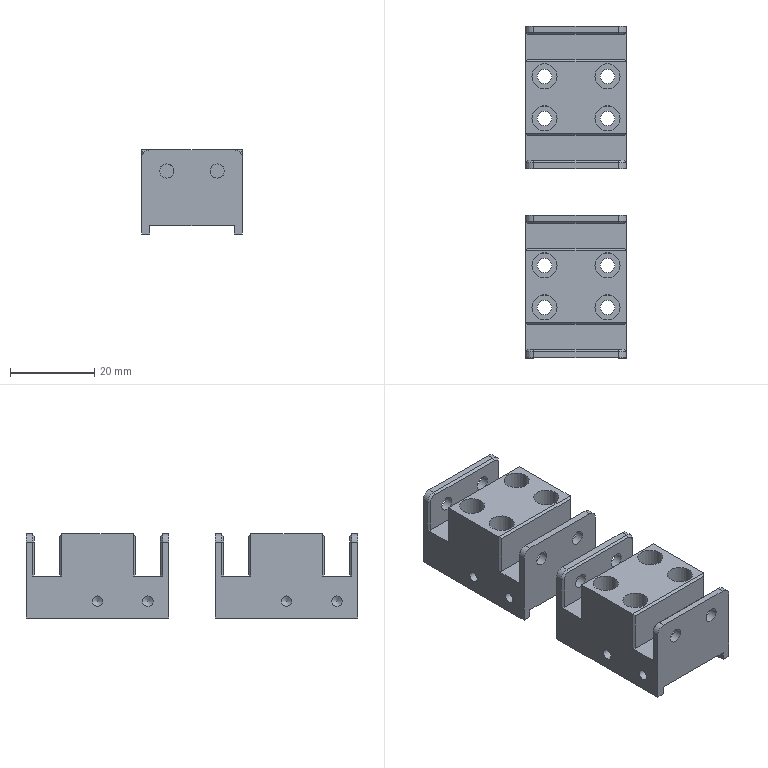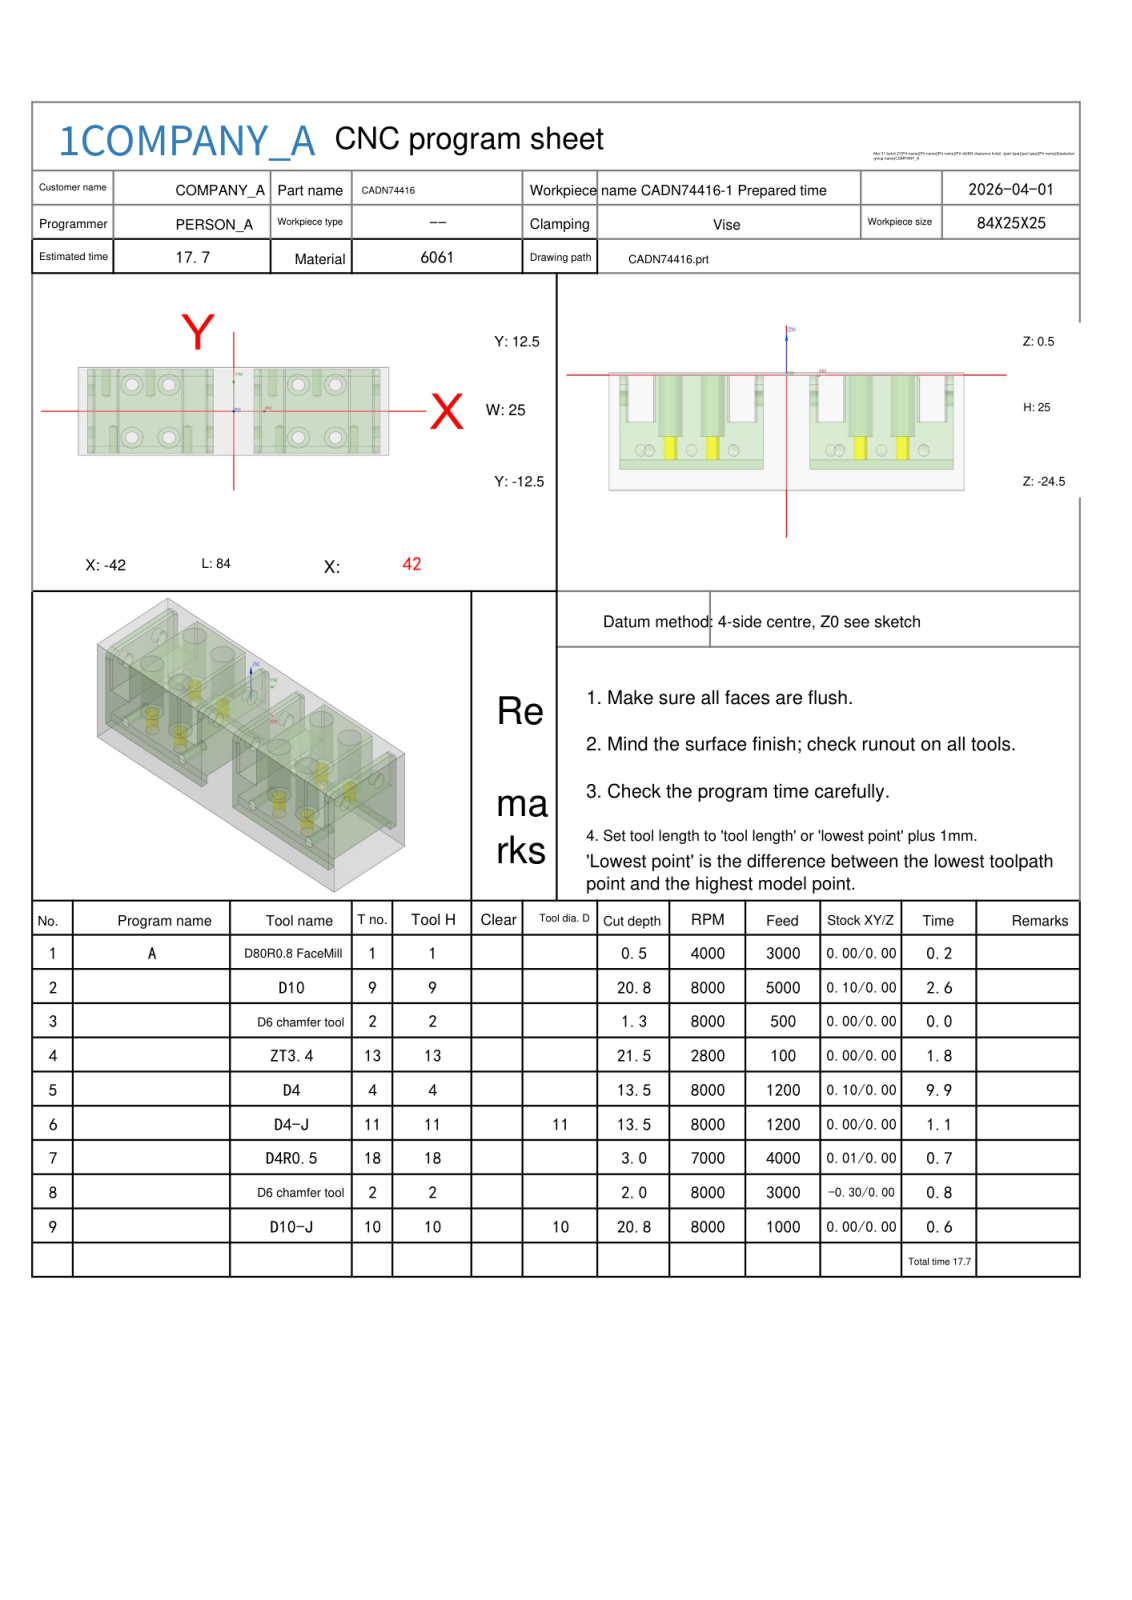NC program | NX | posted by the shop | part box 24 x 79 x 20 mm
Lines 7104 to 7697 of 7697:
N8 T02 M06
(D6 chamfer tool  D=6. R=0. H=02 ce=0.00 di=0.00)
G00 G90 G54 X41.628 Y10.25 M03 S8000
G43 H02 Z20.
M08
Z2.085
G01 Z-1.5 F3000.
G03 X41.328 Y10.33 I-.3 J-.52
X40.808 Y10.03 I0.0 J-.6
G01 X40.8 Y10.
Y-10.
X40.808 Y-10.03
G03 X41.328 Y-10.33 I.52 J.3
X41.628 Y-10.25 I0.0 J.6
G01 Z2.085
G00 Z3.45
X32.171 Y-12.564
Z2.927
G01 Z-1.5
G02 X31. Y-13.3 I-1.171 J.564
G01 X14.
G02 X12.829 Y-12.564 I0.0 J1.3
G01 Z2.927
G00 Z20.
Y12.564
Z2.927
G01 Z-1.5
G02 X14. Y13.3 I1.171 J-.564
G01 X31.
G02 X32.171 Y12.564 I0.0 J-1.3
G01 Z2.927
G00 Z20.
X3.372 Y-10.25
Z2.085
G01 Z-1.5
G03 X3.672 Y-10.33 I.3 J.52
X4.192 Y-10.03 I0.0 J.6
G01 X4.2 Y-10.
Y10.
X4.192 Y10.03
G03 X3.672 Y10.33 I-.52 J-.3
X3.372 Y10.25 I0.0 J-.6
G01 Z2.085
G00 Z2.25
X-3.372
Z2.085
G01 Z-1.5
G03 X-3.672 Y10.33 I-.3 J-.52
X-4.192 Y10.03 I0.0 J-.6
G01 X-4.2 Y10.
Y-10.
X-4.192 Y-10.03
G03 X-3.672 Y-10.33 I.52 J.3
X-3.372 Y-10.25 I0.0 J.6
G01 Z2.085
G00 Z3.45
X-12.829 Y-12.564
Z2.927
G01 Z-1.5
G02 X-14. Y-13.3 I-1.171 J.564
G01 X-31.
G02 X-32.171 Y-12.564 I0.0 J1.3
G01 Z2.927
G00 Z20.
Y12.564
Z2.927
G01 Z-1.5
G02 X-31. Y13.3 I1.171 J-.564
G01 X-14.
G02 X-12.829 Y12.564 I0.0 J-1.3
G01 Z2.927
G00 Z20.
X-41.628 Y-10.25
Z2.085
G01 Z-1.5
G03 X-41.328 Y-10.33 I.3 J.52
X-40.808 Y-10.03 I0.0 J.6
G01 X-40.8 Y-10.
Y10.
X-40.808 Y10.03
G03 X-41.328 Y10.33 I-.52 J-.3
X-41.628 Y10.25 I0.0 J-.6
G01 Z2.085
G00 Z20.
G00 G90 X-36.706 Y13.228 M03 S6500
Z20.
Z.3
G01 Z-1.2 F1500.
G03 X-36.8 Y12.763 I1.106 J-.465
G01 Y10.142
G03 X-35.6 Y8.942 I1.2 J0.0
G01 Y11.2
G03 X-36.8 Y10. I0.0 J-1.2
G01 Y-10.
G03 X-35.6 Y-11.2 I1.2 J0.0
G01 Y-8.942
G03 X-36.8 Y-10.142 I0.0 J-1.2
G01 Y-12.763
G03 X-36.706 Y-13.228 I1.2 J0.0
G01 Z.3
G00 Z20.
X-8.294
Z.3
G01 Z-1.2
G03 X-8.2 Y-12.763 I-1.106 J.465
G01 Y-10.142
G03 X-9.4 Y-8.942 I-1.2 J0.0
G01 Y-11.2
G03 X-8.2 Y-10. I0.0 J1.2
G01 Y10.
G03 X-9.4 Y11.2 I-1.2 J0.0
G01 Y8.942
G03 X-8.2 Y10.142 I0.0 J1.2
G01 Y12.763
G03 X-8.294 Y13.228 I-1.2 J0.0
G01 Z.3
G00 Z20.
X8.294
Z.3
G01 Z-1.2
G03 X8.2 Y12.763 I1.106 J-.465
G01 Y10.142
G03 X9.4 Y8.942 I1.2 J0.0
G01 Y11.2
G03 X8.2 Y10. I0.0 J-1.2
G01 Y-10.
G03 X9.4 Y-11.2 I1.2 J0.0
G01 Y-8.942
G03 X8.2 Y-10.142 I0.0 J-1.2
G01 Y-12.763
G03 X8.294 Y-13.228 I1.2 J0.0
G01 Z.3
G00 Z20.
X36.706
Z.3
G01 Z-1.2
G03 X36.8 Y-12.763 I-1.106 J.465
G01 Y-10.142
G03 X35.6 Y-8.942 I-1.2 J0.0
G01 Y-11.2
G03 X36.8 Y-10. I0.0 J1.2
G01 Y10.
G03 X35.6 Y11.2 I-1.2 J0.0
G01 Y8.942
G03 X36.8 Y10.142 I0.0 J1.2
G01 Y12.763
G03 X36.706 Y13.228 I-1.2 J0.0
G01 Z.3
G00 Z20.
G00 G90 X-15.519 Y8.67 M03 S8000
Z20.
Z2.5
G01 X-15.567 Y8.752 Z2.465 F500.
X-15.764 Y9.013 Z2.346
X-15.996 Y9.244 Z2.227
X-16.259 Y9.44 Z2.108
X-16.546 Y9.596 Z1.989
X-16.853 Y9.71 Z1.87
X-17.173 Y9.78 Z1.75
X-17.5 Y9.803 Z1.631
X-17.827 Y9.78 Z1.512
X-18.147 Y9.71 Z1.393
X-18.454 Y9.596 Z1.274
X-18.741 Y9.44 Z1.154
X-19.004 Y9.244 Z1.035
X-19.236 Y9.013 Z.916
X-19.433 Y8.752 Z.797
X-19.551 Y8.548 Z.711
X-19.679 Y8.247 Z.592
X-19.762 Y7.93 Z.473
X-19.801 Y7.605 Z.354
X-19.792 Y7.278 Z.235
X-19.738 Y6.955 Z.115
X-19.638 Y6.643 Z-.004
X-19.494 Y6.349 Z-.123
X-19.311 Y6.077 Z-.242
X-19.091 Y5.835 Z-.361
X-18.839 Y5.626 Z-.48
X-18.559 Y5.455 Z-.6
X-18.259 Y5.326 Z-.719
X-17.943 Y5.24 Z-.838
X-17.618 Y5.2 Z-.957
X-17.5 Z-1.
G03 X-15.2 Y7.5 I0.0 J2.3
X-17.5 Y9.8 I-2.3 J0.0
X-19.8 Y7.5 I0.0 J-2.3
X-17.5 Y5.2 I2.3 J0.0
X-17.004 Y5.254 I0.0 J2.3
G01 Z1.5
G00 Z20.
X-25.519 Y8.67
Z2.5
G01 X-25.567 Y8.752 Z2.465
X-25.764 Y9.013 Z2.346
X-25.996 Y9.244 Z2.227
X-26.259 Y9.44 Z2.108
X-26.546 Y9.596 Z1.989
X-26.853 Y9.71 Z1.87
X-27.173 Y9.78 Z1.75
X-27.5 Y9.803 Z1.631
X-27.827 Y9.78 Z1.512
X-28.147 Y9.71 Z1.393
X-28.454 Y9.596 Z1.274
X-28.741 Y9.44 Z1.154
X-29.004 Y9.244 Z1.035
X-29.236 Y9.013 Z.916
X-29.433 Y8.752 Z.797
X-29.551 Y8.548 Z.711
X-29.679 Y8.247 Z.592
X-29.762 Y7.93 Z.473
X-29.801 Y7.605 Z.354
X-29.792 Y7.278 Z.235
X-29.738 Y6.955 Z.115
X-29.638 Y6.643 Z-.004
X-29.494 Y6.349 Z-.123
X-29.311 Y6.077 Z-.242
X-29.091 Y5.835 Z-.361
X-28.839 Y5.626 Z-.48
X-28.559 Y5.455 Z-.6
X-28.259 Y5.326 Z-.719
X-27.943 Y5.24 Z-.838
X-27.618 Y5.2 Z-.957
X-27.5 Z-1.
G03 X-25.2 Y7.5 I0.0 J2.3
X-27.5 Y9.8 I-2.3 J0.0
X-29.8 Y7.5 I0.0 J-2.3
X-27.5 Y5.2 I2.3 J0.0
X-27.004 Y5.254 I0.0 J2.3
G01 Z1.5
G00 Z20.
X-25.519 Y-6.33
Z2.5
G01 X-25.567 Y-6.248 Z2.465
X-25.764 Y-5.987 Z2.346
X-25.996 Y-5.756 Z2.227
X-26.259 Y-5.56 Z2.108
X-26.546 Y-5.404 Z1.989
X-26.853 Y-5.29 Z1.87
X-27.173 Y-5.22 Z1.75
X-27.5 Y-5.197 Z1.631
X-27.827 Y-5.22 Z1.512
X-28.147 Y-5.29 Z1.393
X-28.454 Y-5.404 Z1.274
X-28.741 Y-5.56 Z1.154
X-29.004 Y-5.756 Z1.035
X-29.236 Y-5.987 Z.916
X-29.433 Y-6.248 Z.797
X-29.551 Y-6.452 Z.711
X-29.679 Y-6.753 Z.592
X-29.762 Y-7.07 Z.473
X-29.801 Y-7.395 Z.354
X-29.792 Y-7.722 Z.235
X-29.738 Y-8.045 Z.115
X-29.638 Y-8.357 Z-.004
X-29.494 Y-8.652 Z-.123
X-29.311 Y-8.923 Z-.242
X-29.091 Y-9.165 Z-.361
X-28.839 Y-9.374 Z-.48
X-28.559 Y-9.545 Z-.6
X-28.259 Y-9.674 Z-.719
X-27.943 Y-9.76 Z-.838
X-27.618 Y-9.8 Z-.957
X-27.5 Z-1.
G03 X-25.2 Y-7.5 I0.0 J2.3
X-27.5 Y-5.2 I-2.3 J0.0
X-29.8 Y-7.5 I0.0 J-2.3
X-27.5 Y-9.8 I2.3 J0.0
X-27.004 Y-9.746 I0.0 J2.3
G01 Z1.5
G00 Z20.
X-15.519 Y-6.33
Z2.5
G01 X-15.567 Y-6.248 Z2.465
X-15.764 Y-5.987 Z2.346
X-15.996 Y-5.756 Z2.227
X-16.259 Y-5.56 Z2.108
X-16.546 Y-5.404 Z1.989
X-16.853 Y-5.29 Z1.87
X-17.173 Y-5.22 Z1.75
X-17.5 Y-5.197 Z1.631
X-17.827 Y-5.22 Z1.512
X-18.147 Y-5.29 Z1.393
X-18.454 Y-5.404 Z1.274
X-18.741 Y-5.56 Z1.154
X-19.004 Y-5.756 Z1.035
X-19.236 Y-5.987 Z.916
X-19.433 Y-6.248 Z.797
X-19.551 Y-6.452 Z.711
X-19.679 Y-6.753 Z.592
X-19.762 Y-7.07 Z.473
X-19.801 Y-7.395 Z.354
X-19.792 Y-7.722 Z.235
X-19.738 Y-8.045 Z.115
X-19.638 Y-8.357 Z-.004
X-19.494 Y-8.652 Z-.123
X-19.311 Y-8.923 Z-.242
X-19.091 Y-9.165 Z-.361
X-18.839 Y-9.374 Z-.48
X-18.559 Y-9.545 Z-.6
X-18.259 Y-9.674 Z-.719
X-17.943 Y-9.76 Z-.838
X-17.618 Y-9.8 Z-.957
X-17.5 Z-1.
G03 X-15.2 Y-7.5 I0.0 J2.3
X-17.5 Y-5.2 I-2.3 J0.0
X-19.8 Y-7.5 I0.0 J-2.3
X-17.5 Y-9.8 I2.3 J0.0
X-17.004 Y-9.746 I0.0 J2.3
G01 Z1.5
G00 Z20.
X19.481 Y-6.33
Z2.5
G01 X19.433 Y-6.248 Z2.465
X19.236 Y-5.987 Z2.346
X19.004 Y-5.756 Z2.227
X18.741 Y-5.56 Z2.108
X18.454 Y-5.404 Z1.989
X18.147 Y-5.29 Z1.87
X17.827 Y-5.22 Z1.75
X17.5 Y-5.197 Z1.631
X17.173 Y-5.22 Z1.512
X16.853 Y-5.29 Z1.393
X16.546 Y-5.404 Z1.274
X16.259 Y-5.56 Z1.154
X15.996 Y-5.756 Z1.035
X15.764 Y-5.987 Z.916
X15.567 Y-6.248 Z.797
X15.449 Y-6.452 Z.711
X15.321 Y-6.753 Z.592
X15.238 Y-7.07 Z.473
X15.199 Y-7.395 Z.354
X15.208 Y-7.722 Z.235
X15.262 Y-8.045 Z.115
X15.362 Y-8.357 Z-.004
X15.506 Y-8.652 Z-.123
X15.689 Y-8.923 Z-.242
X15.909 Y-9.165 Z-.361
X16.161 Y-9.374 Z-.48
X16.441 Y-9.545 Z-.6
X16.741 Y-9.674 Z-.719
X17.057 Y-9.76 Z-.838
X17.382 Y-9.8 Z-.957
X17.5 Z-1.
G03 X19.8 Y-7.5 I0.0 J2.3
X17.5 Y-5.2 I-2.3 J0.0
X15.2 Y-7.5 I0.0 J-2.3
X17.5 Y-9.8 I2.3 J0.0
X17.996 Y-9.746 I0.0 J2.3
G01 Z1.5
G00 Z20.
X29.481 Y-6.33
Z2.5
G01 X29.433 Y-6.248 Z2.465
X29.236 Y-5.987 Z2.346
X29.004 Y-5.756 Z2.227
X28.741 Y-5.56 Z2.108
X28.454 Y-5.404 Z1.989
X28.147 Y-5.29 Z1.87
X27.827 Y-5.22 Z1.75
X27.5 Y-5.197 Z1.631
X27.173 Y-5.22 Z1.512
X26.853 Y-5.29 Z1.393
X26.546 Y-5.404 Z1.274
X26.259 Y-5.56 Z1.154
X25.996 Y-5.756 Z1.035
X25.764 Y-5.987 Z.916
X25.567 Y-6.248 Z.797
X25.449 Y-6.452 Z.711
X25.321 Y-6.753 Z.592
X25.238 Y-7.07 Z.473
X25.199 Y-7.395 Z.354
X25.208 Y-7.722 Z.235
X25.262 Y-8.045 Z.115
X25.362 Y-8.357 Z-.004
X25.506 Y-8.652 Z-.123
X25.689 Y-8.923 Z-.242
X25.909 Y-9.165 Z-.361
X26.161 Y-9.374 Z-.48
X26.441 Y-9.545 Z-.6
X26.741 Y-9.674 Z-.719
X27.057 Y-9.76 Z-.838
X27.382 Y-9.8 Z-.957
X27.5 Z-1.
G03 X29.8 Y-7.5 I0.0 J2.3
X27.5 Y-5.2 I-2.3 J0.0
X25.2 Y-7.5 I0.0 J-2.3
X27.5 Y-9.8 I2.3 J0.0
X27.996 Y-9.746 I0.0 J2.3
G01 Z1.5
G00 Z20.
X29.481 Y8.67
Z2.5
G01 X29.433 Y8.752 Z2.465
X29.236 Y9.013 Z2.346
X29.004 Y9.244 Z2.227
X28.741 Y9.44 Z2.108
X28.454 Y9.596 Z1.989
X28.147 Y9.71 Z1.87
X27.827 Y9.78 Z1.75
X27.5 Y9.803 Z1.631
X27.173 Y9.78 Z1.512
X26.853 Y9.71 Z1.393
X26.546 Y9.596 Z1.274
X26.259 Y9.44 Z1.154
X25.996 Y9.244 Z1.035
X25.764 Y9.013 Z.916
X25.567 Y8.752 Z.797
X25.449 Y8.548 Z.711
X25.321 Y8.247 Z.592
X25.238 Y7.93 Z.473
X25.199 Y7.605 Z.354
X25.208 Y7.278 Z.235
X25.262 Y6.955 Z.115
X25.362 Y6.643 Z-.004
X25.506 Y6.349 Z-.123
X25.689 Y6.077 Z-.242
X25.909 Y5.835 Z-.361
X26.161 Y5.626 Z-.48
X26.441 Y5.455 Z-.6
X26.741 Y5.326 Z-.719
X27.057 Y5.24 Z-.838
X27.382 Y5.2 Z-.957
X27.5 Z-1.
G03 X29.8 Y7.5 I0.0 J2.3
X27.5 Y9.8 I-2.3 J0.0
X25.2 Y7.5 I0.0 J-2.3
X27.5 Y5.2 I2.3 J0.0
X27.996 Y5.254 I0.0 J2.3
G01 Z1.5
G00 Z20.
X19.481 Y8.67
Z2.5
G01 X19.433 Y8.752 Z2.465
X19.236 Y9.013 Z2.346
X19.004 Y9.244 Z2.227
X18.741 Y9.44 Z2.108
X18.454 Y9.596 Z1.989
X18.147 Y9.71 Z1.87
X17.827 Y9.78 Z1.75
X17.5 Y9.803 Z1.631
X17.173 Y9.78 Z1.512
X16.853 Y9.71 Z1.393
X16.546 Y9.596 Z1.274
X16.259 Y9.44 Z1.154
X15.996 Y9.244 Z1.035
X15.764 Y9.013 Z.916
X15.567 Y8.752 Z.797
X15.449 Y8.548 Z.711
X15.321 Y8.247 Z.592
X15.238 Y7.93 Z.473
X15.199 Y7.605 Z.354
X15.208 Y7.278 Z.235
X15.262 Y6.955 Z.115
X15.362 Y6.643 Z-.004
X15.506 Y6.349 Z-.123
X15.689 Y6.077 Z-.242
X15.909 Y5.835 Z-.361
X16.161 Y5.626 Z-.48
X16.441 Y5.455 Z-.6
X16.741 Y5.326 Z-.719
X17.057 Y5.24 Z-.838
X17.382 Y5.2 Z-.957
X17.5 Z-1.
G03 X19.8 Y7.5 I0.0 J2.3
X17.5 Y9.8 I-2.3 J0.0
X15.2 Y7.5 I0.0 J-2.3
X17.5 Y5.2 I2.3 J0.0
X17.996 Y5.254 I0.0 J2.3
G01 Z1.5
G00 Z20.
G00 G90 X33.4 Y15.907 M03 S6500
Z20.
Z.3
G01 Z-1.2 F1500.
G03 X32.2 Y14.707 I0.0 J-1.2
G01 Y-14.707
G03 X33.4 Y-15.907 I1.2 J0.0
G01 Z.3
G00 Z20.
X11.6
Z.3
G01 Z-1.2
G03 X12.8 Y-14.707 I0.0 J1.2
G01 Y14.707
G03 X11.6 Y15.907 I-1.2 J0.0
G01 Z.3
G00 Z20.
X-11.6
Z.3
G01 Z-1.2
G03 X-12.8 Y14.707 I0.0 J-1.2
G01 Y-14.707
G03 X-11.6 Y-15.907 I1.2 J0.0
G01 Z.3
G00 Z20.
X-33.4
Z.3
G01 Z-1.2
G03 X-32.2 Y-14.707 I0.0 J1.2
G01 Y14.707
G03 X-33.4 Y15.907 I-1.2 J0.0
G01 Z.3
G00 Z20.
G91 G28 Z0.0
M05
M09
G91 G28 Z0.0
M01
N9 T10 M06
(D10-J  D=10. R=0. H=10 ce=0.00 di=0.00)
G00 G90 G54 X40.513 Y-18.116 M03 S8000
G43 H10 Z20.
M08
Z-9.65
G01 Z-10.15 F1000.
G41 D10
X40.497 Y-17.917
G03 X39.5 Y-17. I-.997 J-.083
G01 X5.5
G02 X.5 Y-12. I0.0 J5.
G01 Y12.
G02 X5.5 Y17. I5. J0.0
G01 X39.5
G02 X44.5 Y12. I0.0 J-5.
G01 Y-12.
G02 X39.5 Y-17. I-5. J0.0
G01 X39.
G03 X38. Y-18. I0.0 J-1.
G01 G40 Y-18.2
Z-9.65
G00 Z20.
X-21.5
Z-9.65
G01 Z-10.15
G41 D10
Y-18.
G03 X-22.5 Y-17. I-1. J0.0
G01 X-39.5
G02 X-44.5 Y-12. I0.0 J5.
G01 Y12.
G02 X-39.5 Y17. I5. J0.0
G01 X-5.5
G02 X-.5 Y12. I0.0 J-5.
G01 Y-12.
G02 X-5.5 Y-17. I-5. J0.0
G01 X-22.5
X-23.
G03 X-24. Y-18. I0.0 J-1.
G01 G40 Y-18.2
Z-9.65
G00 Z20.
X-4.487 Y-18.116
Z-19.8
G01 Z-20.3
G41 D10
X-4.503 Y-17.917
G03 X-5.5 Y-17. I-.997 J-.083
G01 X-39.5
G02 X-44.5 Y-12. I0.0 J5.
G01 Y12.
G02 X-39.5 Y17. I5. J0.0
G01 X-5.5
G02 X-.5 Y12. I0.0 J-5.
G01 Y-12.
G02 X-5.5 Y-17. I-5. J0.0
G01 X-6.
G03 X-7. Y-18. I0.0 J-1.
G01 G40 Y-18.2
X.351 Y-15.453
G41 D10
X.526 Y-15.356
G03 X1.038 Y-14.483 I-.488 J.873
X.948 Y-14.069 I-1. J0.0
G02 X.5 Y-12. I4.552 J2.069
G01 Y12.
G02 X5.5 Y17. I5. J0.0
G01 X39.5
G02 X44.5 Y12. I0.0 J-5.
G01 Y-12.
G02 X39.5 Y-17. I-5. J0.0
G01 X5.5
G02 X.948 Y-14.069 I0.0 J5.
X.764 Y-13.604 I4.552 J2.069
G03 X-.183 Y-12.925 I-.947 J-.321
X-.504 Y-12.978 I0.0 J-1.
G01 G40 X0.0 Y-14.398
Z-19.8
G00 Z20.
M05
M09
G91 G28 Z0.0
G91 G28 Y0.0
M30
%